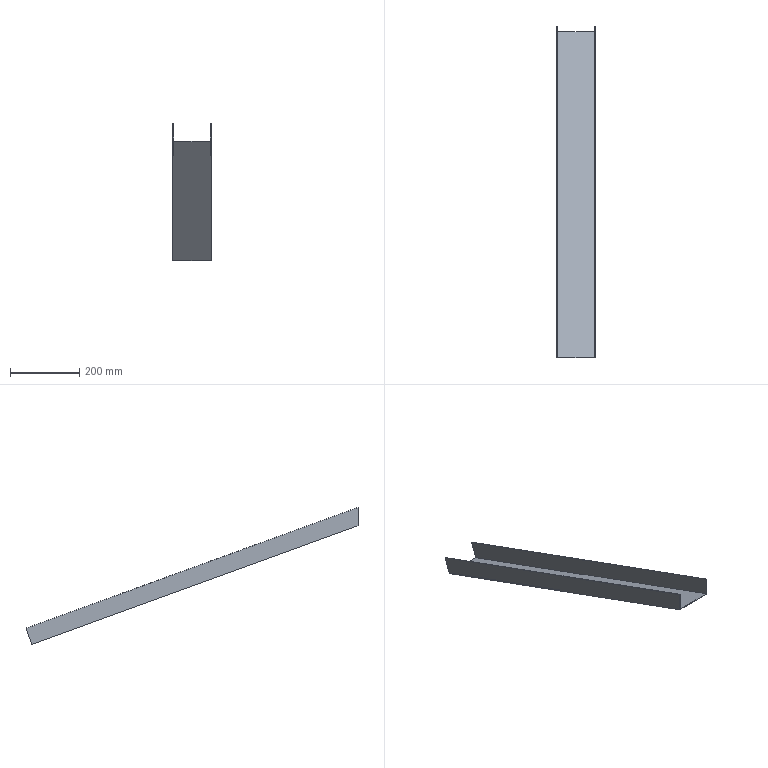Part | NX | features solid 2 | 1 solid | 10 faces | box 110 x 957.101 x 395.341 mm | volume 414032 mm3 | plane 10
STEP:
#1=CARTESIAN_POINT('',(-235.,85.,-47.929));
#2=VERTEX_POINT('',#1);
#3=CARTESIAN_POINT('',(-233.,85.,-47.929));
#4=VERTEX_POINT('',#3);
#5=CARTESIAN_POINT('',(-1135.,85.,-47.929));
#6=DIRECTION('',(1.,0.,0.));
#7=VECTOR('',#6,1000.);
#8=LINE('',#5,#7);
#9=EDGE_CURVE('',#2,#4,#8,.T.);
#10=ORIENTED_EDGE('',*,*,#9,.F.);
#11=CARTESIAN_POINT('',(-235.,85.,-101.138));
#12=VERTEX_POINT('',#11);
#13=CARTESIAN_POINT('',(-235.,85.,40.));
#14=DIRECTION('',(0.,0.,-1.));
#15=VECTOR('',#14,1000.);
#16=LINE('',#13,#15);
#17=EDGE_CURVE('',#2,#12,#16,.T.);
#18=ORIENTED_EDGE('',*,*,#17,.T.);
#19=CARTESIAN_POINT('',(-125.,85.,-101.138));
#20=VERTEX_POINT('',#19);
#21=CARTESIAN_POINT('',(-1135.,85.,-101.138));
#22=DIRECTION('',(1.,0.,0.));
#23=VECTOR('',#22,1000.);
#24=LINE('',#21,#23);
#25=EDGE_CURVE('',#12,#20,#24,.T.);
#26=ORIENTED_EDGE('',*,*,#25,.T.);
#27=CARTESIAN_POINT('',(-125.,85.,-47.929));
#28=VERTEX_POINT('',#27);
#29=CARTESIAN_POINT('',(-125.,85.,-215.937));
#30=DIRECTION('',(0.,0.,-1.));
#31=VECTOR('',#30,1000.);
#32=LINE('',#29,#31);
#33=EDGE_CURVE('',#28,#20,#32,.T.);
#34=ORIENTED_EDGE('',*,*,#33,.F.);
#35=CARTESIAN_POINT('',(-127.,85.,-47.929));
#36=VERTEX_POINT('',#35);
#37=CARTESIAN_POINT('',(-1135.,85.,-47.929));
#38=DIRECTION('',(1.,0.,0.));
#39=VECTOR('',#38,1000.);
#40=LINE('',#37,#39);
#41=EDGE_CURVE('',#36,#28,#40,.T.);
#42=ORIENTED_EDGE('',*,*,#41,.F.);
#43=CARTESIAN_POINT('',(-127.,85.,-99.01));
#44=VERTEX_POINT('',#43);
#45=CARTESIAN_POINT('',(-127.,85.,-215.937));
#46=DIRECTION('',(0.,0.,-1.));
#47=VECTOR('',#46,1000.);
#48=LINE('',#45,#47);
#49=EDGE_CURVE('',#36,#44,#48,.T.);
#50=ORIENTED_EDGE('',*,*,#49,.T.);
#51=CARTESIAN_POINT('',(-233.,85.,-99.01));
#52=VERTEX_POINT('',#51);
#53=CARTESIAN_POINT('',(-1135.,85.,-99.01));
#54=DIRECTION('',(1.,0.,0.));
#55=VECTOR('',#54,1000.);
#56=LINE('',#53,#55);
#57=EDGE_CURVE('',#52,#44,#56,.T.);
#58=ORIENTED_EDGE('',*,*,#57,.F.);
#59=CARTESIAN_POINT('',(-233.,85.,40.));
#60=DIRECTION('',(0.,0.,-1.));
#61=VECTOR('',#60,1000.);
#62=LINE('',#59,#61);
#63=EDGE_CURVE('',#4,#52,#62,.T.);
#64=ORIENTED_EDGE('',*,*,#63,.F.);
#65=EDGE_LOOP('',(#10,#18,#26,#34,#42,#50,#58,#64));
#66=FACE_BOUND('',#65,.T.);
#67=CARTESIAN_POINT('',(-1135.,85.,40.));
#68=DIRECTION('',(0.,-1.,0.));
#69=DIRECTION('',(-1.,0.,0.));
#70=AXIS2_PLACEMENT_3D('',#67,#68,#69);
#71=PLANE('',#70);
#72=ADVANCED_FACE('',(#66),#71,.T.);
#73=CARTESIAN_POINT('',(-125.,1042.101,-396.286));
#74=VERTEX_POINT('',#73);
#75=CARTESIAN_POINT('',(-127.,1042.101,-396.286));
#76=VERTEX_POINT('',#75);
#77=CARTESIAN_POINT('',(-210.,1042.101,-396.286));
#78=DIRECTION('',(-1.,0.,0.));
#79=VECTOR('',#78,1000.);
#80=LINE('',#77,#79);
#81=EDGE_CURVE('',#74,#76,#80,.T.);
#82=ORIENTED_EDGE('',*,*,#81,.F.);
#83=CARTESIAN_POINT('',(-125.,1025.,-443.27));
#84=VERTEX_POINT('',#83);
#85=CARTESIAN_POINT('',(-125.,1042.101,-396.286));
#86=DIRECTION('',(0.,-0.342,-0.9397));
#87=VECTOR('',#86,1000.);
#88=LINE('',#85,#87);
#89=EDGE_CURVE('',#74,#84,#88,.T.);
#90=ORIENTED_EDGE('',*,*,#89,.T.);
#91=CARTESIAN_POINT('',(-235.,1025.,-443.27));
#92=VERTEX_POINT('',#91);
#93=CARTESIAN_POINT('',(-210.,1025.,-443.27));
#94=DIRECTION('',(-1.,0.,0.));
#95=VECTOR('',#94,1000.);
#96=LINE('',#93,#95);
#97=EDGE_CURVE('',#84,#92,#96,.T.);
#98=ORIENTED_EDGE('',*,*,#97,.T.);
#99=CARTESIAN_POINT('',(-235.,1042.101,-396.286));
#100=VERTEX_POINT('',#99);
#101=CARTESIAN_POINT('',(-235.,1042.101,-396.286));
#102=DIRECTION('',(0.,-0.342,-0.9397));
#103=VECTOR('',#102,1000.);
#104=LINE('',#101,#103);
#105=EDGE_CURVE('',#100,#92,#104,.T.);
#106=ORIENTED_EDGE('',*,*,#105,.F.);
#107=CARTESIAN_POINT('',(-233.,1042.101,-396.286));
#108=VERTEX_POINT('',#107);
#109=CARTESIAN_POINT('',(-210.,1042.101,-396.286));
#110=DIRECTION('',(-1.,0.,0.));
#111=VECTOR('',#110,1000.);
#112=LINE('',#109,#111);
#113=EDGE_CURVE('',#108,#100,#112,.T.);
#114=ORIENTED_EDGE('',*,*,#113,.F.);
#115=CARTESIAN_POINT('',(-233.,1025.684,-441.391));
#116=VERTEX_POINT('',#115);
#117=CARTESIAN_POINT('',(-233.,1042.101,-396.286));
#118=DIRECTION('',(0.,-0.342,-0.9397));
#119=VECTOR('',#118,1000.);
#120=LINE('',#117,#119);
#121=EDGE_CURVE('',#108,#116,#120,.T.);
#122=ORIENTED_EDGE('',*,*,#121,.T.);
#123=CARTESIAN_POINT('',(-127.,1025.684,-441.391));
#124=VERTEX_POINT('',#123);
#125=CARTESIAN_POINT('',(-210.,1025.684,-441.391));
#126=DIRECTION('',(-1.,0.,0.));
#127=VECTOR('',#126,1000.);
#128=LINE('',#125,#127);
#129=EDGE_CURVE('',#124,#116,#128,.T.);
#130=ORIENTED_EDGE('',*,*,#129,.F.);
#131=CARTESIAN_POINT('',(-127.,1042.101,-396.286));
#132=DIRECTION('',(0.,-0.342,-0.9397));
#133=VECTOR('',#132,1000.);
#134=LINE('',#131,#133);
#135=EDGE_CURVE('',#76,#124,#134,.T.);
#136=ORIENTED_EDGE('',*,*,#135,.F.);
#137=EDGE_LOOP('',(#82,#90,#98,#106,#114,#122,#130,#136));
#138=FACE_BOUND('',#137,.T.);
#139=CARTESIAN_POINT('',(-210.,1042.101,-396.286));
#140=DIRECTION('',(0.,0.9397,-0.342));
#141=DIRECTION('',(0.,-0.342,-0.9397));
#142=AXIS2_PLACEMENT_3D('',#139,#140,#141);
#143=PLANE('',#142);
#144=ADVANCED_FACE('',(#138),#143,.T.);
#145=ORIENTED_EDGE('',*,*,#113,.T.);
#146=CARTESIAN_POINT('',(-235.,546.597,-215.937));
#147=DIRECTION('',(0.,-0.9397,0.342));
#148=VECTOR('',#147,1000.);
#149=LINE('',#146,#148);
#150=EDGE_CURVE('',#100,#2,#149,.T.);
#151=ORIENTED_EDGE('',*,*,#150,.T.);
#152=ORIENTED_EDGE('',*,*,#9,.T.);
#153=CARTESIAN_POINT('',(-233.,546.597,-215.937));
#154=DIRECTION('',(0.,-0.9397,0.342));
#155=VECTOR('',#154,1000.);
#156=LINE('',#153,#155);
#157=EDGE_CURVE('',#108,#4,#156,.T.);
#158=ORIENTED_EDGE('',*,*,#157,.F.);
#159=EDGE_LOOP('',(#145,#151,#152,#158));
#160=FACE_BOUND('',#159,.T.);
#161=CARTESIAN_POINT('',(-210.,546.597,-215.937));
#162=DIRECTION('',(0.,-0.342,-0.9397));
#163=DIRECTION('',(-1.,0.,0.));
#164=AXIS2_PLACEMENT_3D('',#161,#162,#163);
#165=PLANE('',#164);
#166=ADVANCED_FACE('',(#160),#165,.F.);
#167=CARTESIAN_POINT('',(-235.,529.496,-262.921));
#168=DIRECTION('',(0.,-0.9397,0.342));
#169=VECTOR('',#168,1000.);
#170=LINE('',#167,#169);
#171=EDGE_CURVE('',#92,#12,#170,.T.);
#172=ORIENTED_EDGE('',*,*,#171,.T.);
#173=ORIENTED_EDGE('',*,*,#17,.F.);
#174=ORIENTED_EDGE('',*,*,#150,.F.);
#175=ORIENTED_EDGE('',*,*,#105,.T.);
#176=EDGE_LOOP('',(#172,#173,#174,#175));
#177=FACE_BOUND('',#176,.T.);
#178=CARTESIAN_POINT('',(-235.,546.597,-215.937));
#179=DIRECTION('',(-1.,0.,0.));
#180=DIRECTION('',(0.,-0.08716,0.9962));
#181=AXIS2_PLACEMENT_3D('',#178,#179,#180);
#182=PLANE('',#181);
#183=ADVANCED_FACE('',(#177),#182,.T.);
#184=CARTESIAN_POINT('',(-125.,529.496,-262.921));
#185=DIRECTION('',(0.,0.9397,-0.342));
#186=VECTOR('',#185,1000.);
#187=LINE('',#184,#186);
#188=EDGE_CURVE('',#20,#84,#187,.T.);
#189=ORIENTED_EDGE('',*,*,#188,.T.);
#190=ORIENTED_EDGE('',*,*,#89,.F.);
#191=CARTESIAN_POINT('',(-125.,546.597,-215.937));
#192=DIRECTION('',(0.,0.9397,-0.342));
#193=VECTOR('',#192,1000.);
#194=LINE('',#191,#193);
#195=EDGE_CURVE('',#28,#74,#194,.T.);
#196=ORIENTED_EDGE('',*,*,#195,.F.);
#197=ORIENTED_EDGE('',*,*,#33,.T.);
#198=EDGE_LOOP('',(#189,#190,#196,#197));
#199=FACE_BOUND('',#198,.T.);
#200=CARTESIAN_POINT('',(-125.,546.597,-215.937));
#201=DIRECTION('',(1.,0.,0.));
#202=DIRECTION('',(0.,0.08716,-0.9962));
#203=AXIS2_PLACEMENT_3D('',#200,#201,#202);
#204=PLANE('',#203);
#205=ADVANCED_FACE('',(#199),#204,.T.);
#206=ORIENTED_EDGE('',*,*,#41,.T.);
#207=ORIENTED_EDGE('',*,*,#195,.T.);
#208=ORIENTED_EDGE('',*,*,#81,.T.);
#209=CARTESIAN_POINT('',(-127.,546.597,-215.937));
#210=DIRECTION('',(0.,0.9397,-0.342));
#211=VECTOR('',#210,1000.);
#212=LINE('',#209,#211);
#213=EDGE_CURVE('',#36,#76,#212,.T.);
#214=ORIENTED_EDGE('',*,*,#213,.F.);
#215=EDGE_LOOP('',(#206,#207,#208,#214));
#216=FACE_BOUND('',#215,.T.);
#217=CARTESIAN_POINT('',(-210.,546.597,-215.937));
#218=DIRECTION('',(0.,-0.342,-0.9397));
#219=DIRECTION('',(-1.,0.,0.));
#220=AXIS2_PLACEMENT_3D('',#217,#218,#219);
#221=PLANE('',#220);
#222=ADVANCED_FACE('',(#216),#221,.F.);
#223=ORIENTED_EDGE('',*,*,#171,.F.);
#224=ORIENTED_EDGE('',*,*,#97,.F.);
#225=ORIENTED_EDGE('',*,*,#188,.F.);
#226=ORIENTED_EDGE('',*,*,#25,.F.);
#227=EDGE_LOOP('',(#223,#224,#225,#226));
#228=FACE_BOUND('',#227,.T.);
#229=CARTESIAN_POINT('',(-210.,529.496,-262.921));
#230=DIRECTION('',(0.,-0.342,-0.9397));
#231=DIRECTION('',(-1.,0.,0.));
#232=AXIS2_PLACEMENT_3D('',#229,#230,#231);
#233=PLANE('',#232);
#234=ADVANCED_FACE('',(#228),#233,.T.);
#235=CARTESIAN_POINT('',(-233.,530.18,-261.042));
#236=DIRECTION('',(0.,-0.9397,0.342));
#237=VECTOR('',#236,1000.);
#238=LINE('',#235,#237);
#239=EDGE_CURVE('',#116,#52,#238,.T.);
#240=ORIENTED_EDGE('',*,*,#239,.F.);
#241=ORIENTED_EDGE('',*,*,#121,.F.);
#242=ORIENTED_EDGE('',*,*,#157,.T.);
#243=ORIENTED_EDGE('',*,*,#63,.T.);
#244=EDGE_LOOP('',(#240,#241,#242,#243));
#245=FACE_BOUND('',#244,.T.);
#246=CARTESIAN_POINT('',(-233.,546.597,-215.937));
#247=DIRECTION('',(-1.,0.,0.));
#248=DIRECTION('',(0.,-0.08716,0.9962));
#249=AXIS2_PLACEMENT_3D('',#246,#247,#248);
#250=PLANE('',#249);
#251=ADVANCED_FACE('',(#245),#250,.F.);
#252=CARTESIAN_POINT('',(-127.,530.18,-261.042));
#253=DIRECTION('',(0.,0.9397,-0.342));
#254=VECTOR('',#253,1000.);
#255=LINE('',#252,#254);
#256=EDGE_CURVE('',#44,#124,#255,.T.);
#257=ORIENTED_EDGE('',*,*,#256,.F.);
#258=ORIENTED_EDGE('',*,*,#49,.F.);
#259=ORIENTED_EDGE('',*,*,#213,.T.);
#260=ORIENTED_EDGE('',*,*,#135,.T.);
#261=EDGE_LOOP('',(#257,#258,#259,#260));
#262=FACE_BOUND('',#261,.T.);
#263=CARTESIAN_POINT('',(-127.,546.597,-215.937));
#264=DIRECTION('',(1.,0.,0.));
#265=DIRECTION('',(0.,0.08716,-0.9962));
#266=AXIS2_PLACEMENT_3D('',#263,#264,#265);
#267=PLANE('',#266);
#268=ADVANCED_FACE('',(#262),#267,.F.);
#269=ORIENTED_EDGE('',*,*,#239,.T.);
#270=ORIENTED_EDGE('',*,*,#57,.T.);
#271=ORIENTED_EDGE('',*,*,#256,.T.);
#272=ORIENTED_EDGE('',*,*,#129,.T.);
#273=EDGE_LOOP('',(#269,#270,#271,#272));
#274=FACE_BOUND('',#273,.T.);
#275=CARTESIAN_POINT('',(-210.,530.18,-261.042));
#276=DIRECTION('',(0.,-0.342,-0.9397));
#277=DIRECTION('',(-1.,0.,0.));
#278=AXIS2_PLACEMENT_3D('',#275,#276,#277);
#279=PLANE('',#278);
#280=ADVANCED_FACE('',(#274),#279,.F.);
#281=CLOSED_SHELL('',(#72,#144,#166,#183,#205,#222,#234,#251,#268,#280));
#282=MANIFOLD_SOLID_BREP('',#281);
#283=(LENGTH_UNIT()NAMED_UNIT(*)SI_UNIT(.MILLI.,.METRE.));
#284=UNCERTAINTY_MEASURE_WITH_UNIT(LENGTH_MEASURE(0.00001),#283,'','');
#285=(NAMED_UNIT(*)PLANE_ANGLE_UNIT()SI_UNIT($,.RADIAN.));
#286=(NAMED_UNIT(*)SI_UNIT($,.STERADIAN.)SOLID_ANGLE_UNIT());
#287=(GEOMETRIC_REPRESENTATION_CONTEXT(3)GLOBAL_UNCERTAINTY_ASSIGNED_CONTEXT((#284))GLOBAL_UNIT_ASSIGNED_CONTEXT((#283,#285,#286))REPRESENTATION_CONTEXT('',''));
#288=ADVANCED_BREP_SHAPE_REPRESENTATION('',(#282),#287);